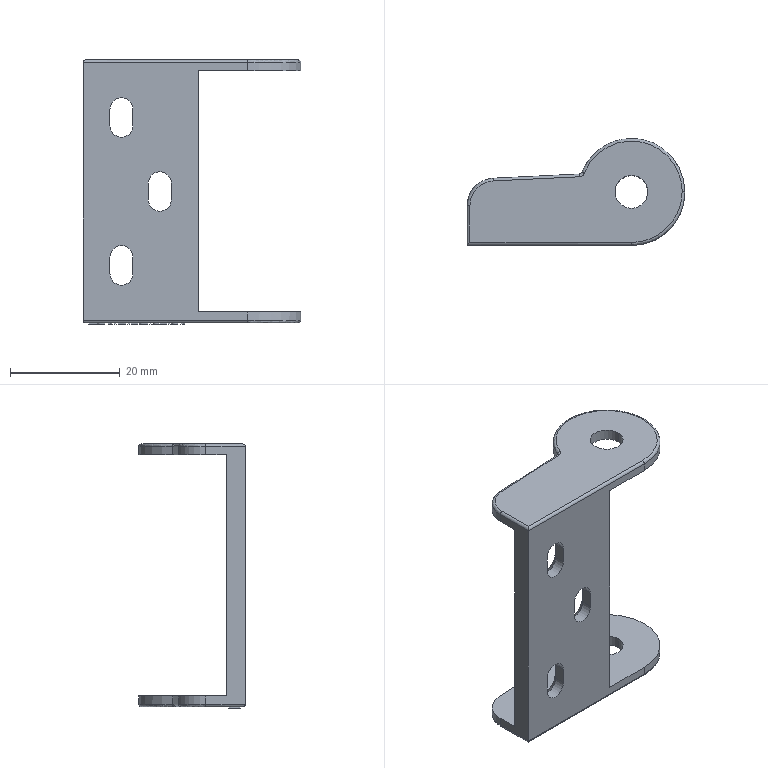Part | STEP file | drag chain fixing head FW175X40-XJT-W3D | 1 solid | 225 faces | box 39.75 x 19.5 x 48.2 mm | volume 4934 mm3 | plane 136 | spline 53 | cylinder 28 | cone 8 | commonest cylinder face diameters 1 x10 4.2 x9 6 x4 19.5 x3 10 x2